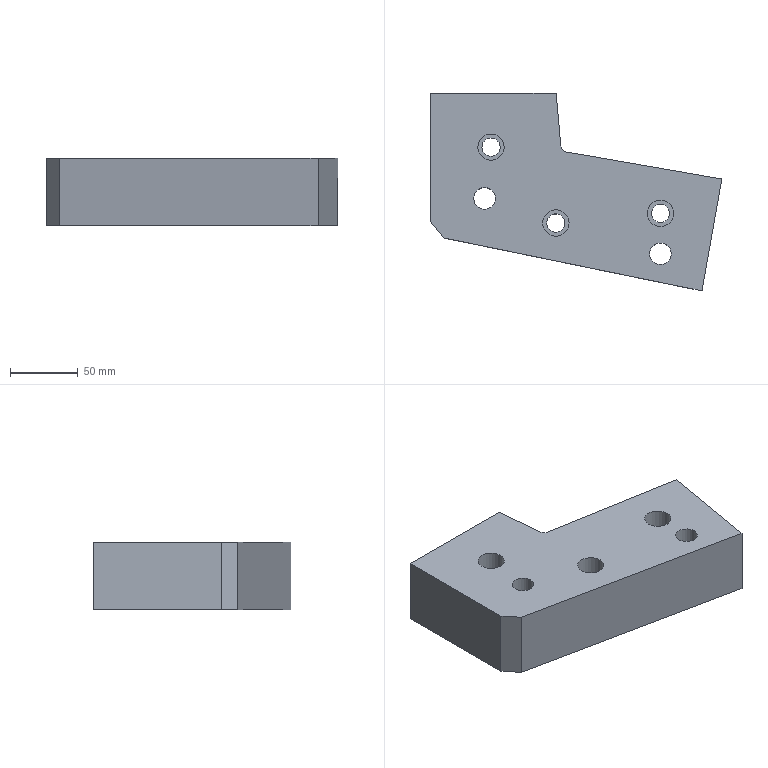Part | NX | features solid 2 | 1 solid | 25 faces | box 215.834 x 146.447 x 50 mm | volume 954922 mm3 | plane 13 | cylinder 10 | spline 2 | commonest cylinder face diameters 13.5 x3 19.5 x3 16 x2 10 x1 14 x1
STEP:
#1=CARTESIAN_POINT('',(903.262,333.786,0.));
#2=VERTEX_POINT('',#1);
#3=CARTESIAN_POINT('',(913.012,333.786,0.));
#4=DIRECTION('',(0.,0.,-1.));
#5=DIRECTION('',(-1.,0.,0.));
#6=AXIS2_PLACEMENT_3D('',#3,#4,#5);
#7=CIRCLE('',#6,9.75);
#8=EDGE_CURVE('',#2,#2,#7,.F.);
#9=ORIENTED_EDGE('',*,*,#8,.F.);
#10=EDGE_LOOP('',(#9));
#11=FACE_BOUND('',#10,.T.);
#12=CARTESIAN_POINT('',(829.797,322.775,0.));
#13=VERTEX_POINT('',#12);
#14=CARTESIAN_POINT('',(1021.231,283.553,0.));
#15=VERTEX_POINT('',#14);
#16=CARTESIAN_POINT('',(1017.086,284.403,0.));
#17=DIRECTION('',(0.9797,-0.2007,0.));
#18=VECTOR('',#17,1000.);
#19=LINE('',#16,#18);
#20=EDGE_CURVE('',#13,#15,#19,.T.);
#21=ORIENTED_EDGE('',*,*,#20,.T.);
#22=CARTESIAN_POINT('',(1035.834,366.376,0.));
#23=VERTEX_POINT('',#22);
#24=CARTESIAN_POINT('',(1025.414,307.279,0.));
#25=DIRECTION('',(0.1736,0.9848,0.));
#26=VECTOR('',#25,1000.);
#27=LINE('',#24,#26);
#28=EDGE_CURVE('',#15,#23,#27,.T.);
#29=ORIENTED_EDGE('',*,*,#28,.T.);
#30=CARTESIAN_POINT('',(920.475,386.408,0.));
#31=VERTEX_POINT('',#30);
#32=CARTESIAN_POINT('',(1323.576,316.335,0.));
#33=CARTESIAN_POINT('',(1303.952,319.748,0.));
#34=CARTESIAN_POINT('',(1284.328,323.16,0.));
#35=CARTESIAN_POINT('',(1264.704,326.573,0.));
#36=CARTESIAN_POINT('',(1233.889,331.932,0.));
#37=CARTESIAN_POINT('',(1172.258,342.651,0.));
#38=CARTESIAN_POINT('',(1095.22,356.049,0.));
#39=CARTESIAN_POINT('',(1033.589,366.767,0.));
#40=CARTESIAN_POINT('',(987.365,374.804,0.));
#41=CARTESIAN_POINT('',(948.847,381.509,0.));
#42=CARTESIAN_POINT('',(923.808,385.853,0.));
#43=CARTESIAN_POINT('',(914.109,387.486,0.));
#44=CARTESIAN_POINT('',(912.091,387.827,0.));
#45=CARTESIAN_POINT('',(911.971,387.848,0.));
#46=CARTESIAN_POINT('',(911.79,387.876,0.));
#47=CARTESIAN_POINT('',(911.394,387.917,0.));
#48=CARTESIAN_POINT('',(910.546,388.022,0.));
#49=CARTESIAN_POINT('',(908.847,388.221,0.));
#50=CARTESIAN_POINT('',(906.42,388.511,0.));
#51=CARTESIAN_POINT('',(903.994,388.799,0.));
#52=CARTESIAN_POINT('',(902.295,389.001,0.));
#53=CARTESIAN_POINT('',(901.446,389.101,0.));
#54=CARTESIAN_POINT('',(901.052,389.148,0.));
#55=CARTESIAN_POINT('',(900.87,389.17,0.));
#56=CARTESIAN_POINT('',(900.748,389.184,0.));
#57=CARTESIAN_POINT('',(899.68,389.239,0.));
#58=CARTESIAN_POINT('',(897.973,389.35,0.));
#59=CARTESIAN_POINT('',(896.023,389.486,0.));
#60=CARTESIAN_POINT('',(894.456,389.561,0.));
#61=CARTESIAN_POINT('',(892.989,389.903,0.));
#62=CARTESIAN_POINT('',(891.495,390.907,0.));
#63=CARTESIAN_POINT('',(890.458,392.378,0.));
#64=CARTESIAN_POINT('',(890.077,393.863,0.));
#65=CARTESIAN_POINT('',(889.825,397.101,0.));
#66=CARTESIAN_POINT('',(889.362,402.393,0.));
#67=CARTESIAN_POINT('',(888.928,407.354,0.));
#68=CARTESIAN_POINT('',(888.696,410.,0.));
#69=CARTESIAN_POINT('',(886.96,429.843,0.));
#70=CARTESIAN_POINT('',(885.224,449.685,0.));
#71=CARTESIAN_POINT('',(883.488,469.528,0.));
#72=B_SPLINE_CURVE_WITH_KNOTS('',3,(#32,#33,#34,#35,#36,#37,#38,#39,#40,#41,#42,#43,#44,#45,#46,#47,#48,#49,#50,#51,#52,#53,#54,#55,#56,#57,#58,#59,#60,#61,#62,#63,#64,#65,#66,#67,#68,#69,#70,#71),.UNSPECIFIED.,.F.,.F.,(4,3,1,1,1,1,1,1,1,1,1,1,1,1,1,1,1,1,1,1,1,1,1,1,1,1,1,1,1,1,1,1,3,4),(-0.15,0.,0.2355,0.4711,0.5889,0.7066,0.8244,0.8833,0.898,0.8985,0.8987,0.8989,0.8999,0.9017,0.9054,0.9127,0.9201,0.9238,0.9256,0.9265,0.9268,0.927,0.9275,0.9348,0.9399,0.9422,0.9466,0.9511,0.9555,0.96,0.9625,0.98,1.,1.15),.UNSPECIFIED.);
#73=EDGE_CURVE('',#23,#31,#72,.T.);
#74=ORIENTED_EDGE('',*,*,#73,.T.);
#75=CARTESIAN_POINT('',(916.651,390.837,0.));
#76=VERTEX_POINT('',#75);
#77=CARTESIAN_POINT('',(921.632,391.273,0.));
#78=DIRECTION('',(0.,0.,-1.));
#79=DIRECTION('',(-1.,0.,0.));
#80=AXIS2_PLACEMENT_3D('',#77,#78,#79);
#81=CIRCLE('',#80,5.);
#82=EDGE_CURVE('',#31,#76,#81,.T.);
#83=ORIENTED_EDGE('',*,*,#82,.T.);
#84=CARTESIAN_POINT('',(913.224,430.,0.));
#85=VERTEX_POINT('',#84);
#86=CARTESIAN_POINT('',(916.651,390.837,0.));
#87=DIRECTION('',(-0.08716,0.9962,0.));
#88=VECTOR('',#87,1000.);
#89=LINE('',#86,#88);
#90=EDGE_CURVE('',#76,#85,#89,.T.);
#91=ORIENTED_EDGE('',*,*,#90,.T.);
#92=CARTESIAN_POINT('',(820.,430.,0.));
#93=VERTEX_POINT('',#92);
#94=CARTESIAN_POINT('',(1021.9,430.,0.));
#95=DIRECTION('',(1.,0.,0.));
#96=VECTOR('',#95,1000.);
#97=LINE('',#94,#96);
#98=EDGE_CURVE('',#85,#93,#97,.F.);
#99=ORIENTED_EDGE('',*,*,#98,.T.);
#100=CARTESIAN_POINT('',(820.,334.782,0.));
#101=VERTEX_POINT('',#100);
#102=CARTESIAN_POINT('',(820.,410.,0.));
#103=DIRECTION('',(0.,-1.,0.));
#104=VECTOR('',#103,1000.);
#105=LINE('',#102,#104);
#106=EDGE_CURVE('',#93,#101,#105,.T.);
#107=ORIENTED_EDGE('',*,*,#106,.T.);
#108=CARTESIAN_POINT('',(820.,334.782,0.));
#109=DIRECTION('',(-0.6322,0.7748,0.));
#110=VECTOR('',#109,1000.);
#111=LINE('',#108,#110);
#112=EDGE_CURVE('',#101,#13,#111,.F.);
#113=ORIENTED_EDGE('',*,*,#112,.T.);
#114=EDGE_LOOP('',(#21,#29,#74,#83,#91,#99,#107,#113));
#115=FACE_BOUND('',#114,.T.);
#116=CARTESIAN_POINT('',(980.711,340.91,0.));
#117=VERTEX_POINT('',#116);
#118=CARTESIAN_POINT('',(990.461,340.91,0.));
#119=DIRECTION('',(0.,0.,-1.));
#120=DIRECTION('',(-1.,0.,0.));
#121=AXIS2_PLACEMENT_3D('',#118,#119,#120);
#122=CIRCLE('',#121,9.75);
#123=EDGE_CURVE('',#117,#117,#122,.F.);
#124=ORIENTED_EDGE('',*,*,#123,.F.);
#125=EDGE_LOOP('',(#124));
#126=FACE_BOUND('',#125,.T.);
#127=CARTESIAN_POINT('',(855.25,390.,0.));
#128=VERTEX_POINT('',#127);
#129=CARTESIAN_POINT('',(865.,390.,0.));
#130=DIRECTION('',(0.,0.,-1.));
#131=DIRECTION('',(-1.,0.,0.));
#132=AXIS2_PLACEMENT_3D('',#129,#130,#131);
#133=CIRCLE('',#132,9.75);
#134=EDGE_CURVE('',#128,#128,#133,.F.);
#135=ORIENTED_EDGE('',*,*,#134,.F.);
#136=EDGE_LOOP('',(#135));
#137=FACE_BOUND('',#136,.T.);
#138=CARTESIAN_POINT('',(852.203,352.007,0.));
#139=VERTEX_POINT('',#138);
#140=CARTESIAN_POINT('',(860.203,352.007,0.));
#141=DIRECTION('',(0.,0.,-1.));
#142=DIRECTION('',(-1.,0.,0.));
#143=AXIS2_PLACEMENT_3D('',#140,#141,#142);
#144=CIRCLE('',#143,8.);
#145=EDGE_CURVE('',#139,#139,#144,.F.);
#146=ORIENTED_EDGE('',*,*,#145,.F.);
#147=EDGE_LOOP('',(#146));
#148=FACE_BOUND('',#147,.T.);
#149=CARTESIAN_POINT('',(982.461,310.91,0.));
#150=VERTEX_POINT('',#149);
#151=CARTESIAN_POINT('',(990.461,310.91,0.));
#152=DIRECTION('',(0.,0.,-1.));
#153=DIRECTION('',(-1.,0.,0.));
#154=AXIS2_PLACEMENT_3D('',#151,#152,#153);
#155=CIRCLE('',#154,8.);
#156=EDGE_CURVE('',#150,#150,#155,.F.);
#157=ORIENTED_EDGE('',*,*,#156,.F.);
#158=EDGE_LOOP('',(#157));
#159=FACE_BOUND('',#158,.T.);
#160=CARTESIAN_POINT('',(1021.9,307.899,0.));
#161=DIRECTION('',(0.,0.,-1.));
#162=DIRECTION('',(1.,0.,0.));
#163=AXIS2_PLACEMENT_3D('',#160,#161,#162);
#164=PLANE('',#163);
#165=ADVANCED_FACE('',(#11,#115,#126,#137,#148,#159),#164,.F.);
#166=CARTESIAN_POINT('',(852.203,352.007,-50.));
#167=VERTEX_POINT('',#166);
#168=CARTESIAN_POINT('',(860.203,352.007,-50.));
#169=DIRECTION('',(0.,0.,-1.));
#170=DIRECTION('',(-1.,0.,0.));
#171=AXIS2_PLACEMENT_3D('',#168,#169,#170);
#172=CIRCLE('',#171,8.);
#173=EDGE_CURVE('',#167,#167,#172,.F.);
#174=ORIENTED_EDGE('',*,*,#173,.T.);
#175=EDGE_LOOP('',(#174));
#176=FACE_BOUND('',#175,.T.);
#177=CARTESIAN_POINT('',(858.25,390.,-50.));
#178=VERTEX_POINT('',#177);
#179=CARTESIAN_POINT('',(865.,390.,-50.));
#180=DIRECTION('',(0.,0.,-1.));
#181=DIRECTION('',(-1.,0.,0.));
#182=AXIS2_PLACEMENT_3D('',#179,#180,#181);
#183=CIRCLE('',#182,6.75);
#184=EDGE_CURVE('',#178,#178,#183,.F.);
#185=ORIENTED_EDGE('',*,*,#184,.T.);
#186=EDGE_LOOP('',(#185));
#187=FACE_BOUND('',#186,.T.);
#188=CARTESIAN_POINT('',(983.711,340.91,-50.));
#189=VERTEX_POINT('',#188);
#190=CARTESIAN_POINT('',(990.461,340.91,-50.));
#191=DIRECTION('',(0.,0.,-1.));
#192=DIRECTION('',(-1.,0.,0.));
#193=AXIS2_PLACEMENT_3D('',#190,#191,#192);
#194=CIRCLE('',#193,6.75);
#195=EDGE_CURVE('',#189,#189,#194,.F.);
#196=ORIENTED_EDGE('',*,*,#195,.T.);
#197=EDGE_LOOP('',(#196));
#198=FACE_BOUND('',#197,.T.);
#199=CARTESIAN_POINT('',(1021.231,283.553,-50.));
#200=VERTEX_POINT('',#199);
#201=CARTESIAN_POINT('',(1035.487,364.407,-50.));
#202=VERTEX_POINT('',#201);
#203=CARTESIAN_POINT('',(1025.414,307.279,-50.));
#204=DIRECTION('',(0.1736,0.9848,0.));
#205=VECTOR('',#204,1000.);
#206=LINE('',#203,#205);
#207=EDGE_CURVE('',#200,#202,#206,.T.);
#208=ORIENTED_EDGE('',*,*,#207,.F.);
#209=CARTESIAN_POINT('',(829.797,322.775,-50.));
#210=VERTEX_POINT('',#209);
#211=CARTESIAN_POINT('',(1017.086,284.403,-50.));
#212=DIRECTION('',(0.9797,-0.2007,0.));
#213=VECTOR('',#212,1000.);
#214=LINE('',#211,#213);
#215=EDGE_CURVE('',#210,#200,#214,.T.);
#216=ORIENTED_EDGE('',*,*,#215,.F.);
#217=CARTESIAN_POINT('',(820.,334.782,-50.));
#218=VERTEX_POINT('',#217);
#219=CARTESIAN_POINT('',(913.856,219.747,-50.));
#220=DIRECTION('',(0.6322,-0.7748,0.));
#221=VECTOR('',#220,1000.);
#222=LINE('',#219,#221);
#223=EDGE_CURVE('',#210,#218,#222,.F.);
#224=ORIENTED_EDGE('',*,*,#223,.T.);
#225=CARTESIAN_POINT('',(820.,430.,-50.));
#226=VERTEX_POINT('',#225);
#227=CARTESIAN_POINT('',(820.,410.,-50.));
#228=DIRECTION('',(0.,-1.,0.));
#229=VECTOR('',#228,1000.);
#230=LINE('',#227,#229);
#231=EDGE_CURVE('',#226,#218,#230,.T.);
#232=ORIENTED_EDGE('',*,*,#231,.F.);
#233=CARTESIAN_POINT('',(911.217,430.,-50.));
#234=VERTEX_POINT('',#233);
#235=CARTESIAN_POINT('',(1021.9,430.,-50.));
#236=DIRECTION('',(1.,0.,0.));
#237=VECTOR('',#236,1000.);
#238=LINE('',#235,#237);
#239=EDGE_CURVE('',#234,#226,#238,.F.);
#240=ORIENTED_EDGE('',*,*,#239,.F.);
#241=CARTESIAN_POINT('',(914.658,390.663,-50.));
#242=VERTEX_POINT('',#241);
#243=CARTESIAN_POINT('',(914.658,390.663,-50.));
#244=DIRECTION('',(-0.08716,0.9962,0.));
#245=VECTOR('',#244,1000.);
#246=LINE('',#243,#245);
#247=EDGE_CURVE('',#242,#234,#246,.T.);
#248=ORIENTED_EDGE('',*,*,#247,.F.);
#249=CARTESIAN_POINT('',(920.081,384.447,-50.));
#250=VERTEX_POINT('',#249);
#251=CARTESIAN_POINT('',(921.632,391.273,-50.));
#252=DIRECTION('',(0.,0.,-1.));
#253=DIRECTION('',(-1.,0.,0.));
#254=AXIS2_PLACEMENT_3D('',#251,#252,#253);
#255=CIRCLE('',#254,7.);
#256=EDGE_CURVE('',#250,#242,#255,.T.);
#257=ORIENTED_EDGE('',*,*,#256,.F.);
#258=CARTESIAN_POINT('',(920.081,384.447,-50.));
#259=CARTESIAN_POINT('',(920.552,384.367,-50.));
#260=CARTESIAN_POINT('',(921.288,384.241,-50.));
#261=CARTESIAN_POINT('',(922.185,384.088,-50.));
#262=CARTESIAN_POINT('',(922.726,383.995,-50.));
#263=CARTESIAN_POINT('',(923.034,383.943,-50.));
#264=CARTESIAN_POINT('',(923.367,383.886,-50.));
#265=CARTESIAN_POINT('',(923.396,383.881,-50.));
#266=CARTESIAN_POINT('',(923.576,383.85,-50.));
#267=CARTESIAN_POINT('',(923.851,383.803,-50.));
#268=CARTESIAN_POINT('',(924.31,383.724,-50.));
#269=CARTESIAN_POINT('',(924.87,383.628,-50.));
#270=CARTESIAN_POINT('',(925.66,383.492,-50.));
#271=CARTESIAN_POINT('',(926.718,383.31,-50.));
#272=CARTESIAN_POINT('',(928.103,383.072,-50.));
#273=CARTESIAN_POINT('',(930.103,382.726,-50.));
#274=CARTESIAN_POINT('',(932.889,382.245,-50.));
#275=CARTESIAN_POINT('',(936.692,381.586,-50.));
#276=CARTESIAN_POINT('',(940.241,380.97,-50.));
#277=CARTESIAN_POINT('',(943.314,380.437,-50.));
#278=CARTESIAN_POINT('',(945.322,380.088,-50.));
#279=CARTESIAN_POINT('',(946.793,379.833,-50.));
#280=CARTESIAN_POINT('',(947.521,379.706,-50.));
#281=CARTESIAN_POINT('',(947.972,379.628,-50.));
#282=CARTESIAN_POINT('',(948.365,379.56,-50.));
#283=CARTESIAN_POINT('',(949.073,379.437,-50.));
#284=CARTESIAN_POINT('',(950.244,379.233,-50.));
#285=CARTESIAN_POINT('',(951.737,378.974,-50.));
#286=CARTESIAN_POINT('',(954.11,378.561,-50.));
#287=CARTESIAN_POINT('',(957.082,378.045,-50.));
#288=CARTESIAN_POINT('',(960.645,377.425,-50.));
#289=CARTESIAN_POINT('',(965.397,376.599,-50.));
#290=CARTESIAN_POINT('',(971.337,375.567,-50.));
#291=CARTESIAN_POINT('',(978.465,374.327,-50.));
#292=CARTESIAN_POINT('',(985.593,373.088,-50.));
#293=CARTESIAN_POINT('',(995.097,371.435,-50.));
#294=CARTESIAN_POINT('',(1006.976,369.369,-50.));
#295=CARTESIAN_POINT('',(1021.232,366.889,-50.));
#296=CARTESIAN_POINT('',(1030.736,365.235,-50.));
#297=CARTESIAN_POINT('',(1035.487,364.408,-50.));
#298=B_SPLINE_CURVE_WITH_KNOTS('',3,(#258,#259,#260,#261,#262,#263,#264,#265,#266,#267,#268,#269,#270,#271,#272,#273,#274,#275,#276,#277,#278,#279,#280,#281,#282,#283,#284,#285,#286,#287,#288,#289,#290,#291,#292,#293,#294,#295,#296,#297),.UNSPECIFIED.,.F.,.F.,(4,1,1,1,1,1,1,1,1,1,1,1,1,1,1,1,1,1,1,1,1,1,1,1,1,1,1,1,1,1,1,1,1,1,1,1,1,4),(0.1827,0.1849,0.1861,0.1866,0.1872,0.1875,0.1878,0.1883,0.1895,0.1917,0.194,0.1963,0.2008,0.2053,0.2099,0.2189,0.228,0.237,0.2416,0.2461,0.2484,0.2495,0.2501,0.2506,0.2529,0.2551,0.2597,0.2642,0.2733,0.2823,0.2914,0.3095,0.3276,0.3457,0.3639,0.4001,0.4363,0.4726),.UNSPECIFIED.);
#299=EDGE_CURVE('',#202,#250,#298,.F.);
#300=ORIENTED_EDGE('',*,*,#299,.F.);
#301=EDGE_LOOP('',(#208,#216,#224,#232,#240,#248,#257,#300));
#302=FACE_BOUND('',#301,.T.);
#303=CARTESIAN_POINT('',(906.262,333.786,-50.));
#304=VERTEX_POINT('',#303);
#305=CARTESIAN_POINT('',(913.012,333.786,-50.));
#306=DIRECTION('',(0.,0.,-1.));
#307=DIRECTION('',(-1.,0.,0.));
#308=AXIS2_PLACEMENT_3D('',#305,#306,#307);
#309=CIRCLE('',#308,6.75);
#310=EDGE_CURVE('',#304,#304,#309,.T.);
#311=ORIENTED_EDGE('',*,*,#310,.F.);
#312=EDGE_LOOP('',(#311));
#313=FACE_BOUND('',#312,.T.);
#314=CARTESIAN_POINT('',(982.461,310.91,-50.));
#315=VERTEX_POINT('',#314);
#316=CARTESIAN_POINT('',(990.461,310.91,-50.));
#317=DIRECTION('',(0.,0.,-1.));
#318=DIRECTION('',(-1.,0.,0.));
#319=AXIS2_PLACEMENT_3D('',#316,#317,#318);
#320=CIRCLE('',#319,8.);
#321=EDGE_CURVE('',#315,#315,#320,.F.);
#322=ORIENTED_EDGE('',*,*,#321,.T.);
#323=EDGE_LOOP('',(#322));
#324=FACE_BOUND('',#323,.T.);
#325=CARTESIAN_POINT('',(1021.9,307.899,-50.));
#326=DIRECTION('',(0.,0.,-1.));
#327=DIRECTION('',(1.,0.,0.));
#328=AXIS2_PLACEMENT_3D('',#325,#326,#327);
#329=PLANE('',#328);
#330=ADVANCED_FACE('',(#176,#187,#198,#302,#313,#324),#329,.T.);
#331=ORIENTED_EDGE('',*,*,#310,.T.);
#332=EDGE_LOOP('',(#331));
#333=FACE_BOUND('',#332,.T.);
#334=CARTESIAN_POINT('',(919.762,333.786,-25.));
#335=VERTEX_POINT('',#334);
#336=CARTESIAN_POINT('',(913.012,333.786,-25.));
#337=DIRECTION('',(0.,0.,1.));
#338=DIRECTION('',(1.,0.,0.));
#339=AXIS2_PLACEMENT_3D('',#336,#337,#338);
#340=CIRCLE('',#339,6.75);
#341=EDGE_CURVE('',#335,#335,#340,.F.);
#342=ORIENTED_EDGE('',*,*,#341,.F.);
#343=EDGE_LOOP('',(#342));
#344=FACE_BOUND('',#343,.T.);
#345=CARTESIAN_POINT('',(913.012,333.786,-15.));
#346=DIRECTION('',(0.,0.,-1.));
#347=DIRECTION('',(-1.,0.,0.));
#348=AXIS2_PLACEMENT_3D('',#345,#346,#347);
#349=CYLINDRICAL_SURFACE('',#348,6.75);
#350=ADVANCED_FACE('',(#333,#344),#349,.F.);
#351=CARTESIAN_POINT('',(874.75,390.,-25.));
#352=VERTEX_POINT('',#351);
#353=CARTESIAN_POINT('',(865.,390.,-25.));
#354=DIRECTION('',(0.,0.,1.));
#355=DIRECTION('',(1.,0.,0.));
#356=AXIS2_PLACEMENT_3D('',#353,#354,#355);
#357=CIRCLE('',#356,9.75);
#358=EDGE_CURVE('',#352,#352,#357,.T.);
#359=ORIENTED_EDGE('',*,*,#358,.T.);
#360=EDGE_LOOP('',(#359));
#361=FACE_BOUND('',#360,.T.);
#362=CARTESIAN_POINT('',(871.75,390.,-25.));
#363=VERTEX_POINT('',#362);
#364=CARTESIAN_POINT('',(865.,390.,-25.));
#365=DIRECTION('',(0.,0.,1.));
#366=DIRECTION('',(1.,0.,0.));
#367=AXIS2_PLACEMENT_3D('',#364,#365,#366);
#368=CIRCLE('',#367,6.75);
#369=EDGE_CURVE('',#363,#363,#368,.F.);
#370=ORIENTED_EDGE('',*,*,#369,.T.);
#371=EDGE_LOOP('',(#370));
#372=FACE_BOUND('',#371,.T.);
#373=CARTESIAN_POINT('',(865.,390.,-25.));
#374=DIRECTION('',(0.,0.,1.));
#375=DIRECTION('',(1.,0.,0.));
#376=AXIS2_PLACEMENT_3D('',#373,#374,#375);
#377=PLANE('',#376);
#378=ADVANCED_FACE('',(#361,#372),#377,.T.);
#379=CARTESIAN_POINT('',(1000.211,340.91,-25.));
#380=VERTEX_POINT('',#379);
#381=CARTESIAN_POINT('',(990.461,340.91,-25.));
#382=DIRECTION('',(0.,0.,1.));
#383=DIRECTION('',(1.,0.,0.));
#384=AXIS2_PLACEMENT_3D('',#381,#382,#383);
#385=CIRCLE('',#384,9.75);
#386=EDGE_CURVE('',#380,#380,#385,.T.);
#387=ORIENTED_EDGE('',*,*,#386,.T.);
#388=EDGE_LOOP('',(#387));
#389=FACE_BOUND('',#388,.T.);
#390=CARTESIAN_POINT('',(997.211,340.91,-25.));
#391=VERTEX_POINT('',#390);
#392=CARTESIAN_POINT('',(990.461,340.91,-25.));
#393=DIRECTION('',(0.,0.,1.));
#394=DIRECTION('',(1.,0.,0.));
#395=AXIS2_PLACEMENT_3D('',#392,#393,#394);
#396=CIRCLE('',#395,6.75);
#397=EDGE_CURVE('',#391,#391,#396,.F.);
#398=ORIENTED_EDGE('',*,*,#397,.T.);
#399=EDGE_LOOP('',(#398));
#400=FACE_BOUND('',#399,.T.);
#401=CARTESIAN_POINT('',(990.461,340.91,-25.));
#402=DIRECTION('',(0.,0.,1.));
#403=DIRECTION('',(1.,0.,0.));
#404=AXIS2_PLACEMENT_3D('',#401,#402,#403);
#405=PLANE('',#404);
#406=ADVANCED_FACE('',(#389,#400),#405,.T.);
#407=ORIENTED_EDGE('',*,*,#184,.F.);
#408=EDGE_LOOP('',(#407));
#409=FACE_BOUND('',#408,.T.);
#410=ORIENTED_EDGE('',*,*,#369,.F.);
#411=EDGE_LOOP('',(#410));
#412=FACE_BOUND('',#411,.T.);
#413=CARTESIAN_POINT('',(865.,390.,75.));
#414=DIRECTION('',(0.,0.,-1.));
#415=DIRECTION('',(-1.,0.,0.));
#416=AXIS2_PLACEMENT_3D('',#413,#414,#415);
#417=CYLINDRICAL_SURFACE('',#416,6.75);
#418=ADVANCED_FACE('',(#409,#412),#417,.F.);
#419=ORIENTED_EDGE('',*,*,#195,.F.);
#420=EDGE_LOOP('',(#419));
#421=FACE_BOUND('',#420,.T.);
#422=ORIENTED_EDGE('',*,*,#397,.F.);
#423=EDGE_LOOP('',(#422));
#424=FACE_BOUND('',#423,.T.);
#425=CARTESIAN_POINT('',(990.461,340.91,75.));
#426=DIRECTION('',(0.,0.,-1.));
#427=DIRECTION('',(-1.,0.,0.));
#428=AXIS2_PLACEMENT_3D('',#425,#426,#427);
#429=CYLINDRICAL_SURFACE('',#428,6.75);
#430=ADVANCED_FACE('',(#421,#424),#429,.F.);
#431=ORIENTED_EDGE('',*,*,#173,.F.);
#432=EDGE_LOOP('',(#431));
#433=FACE_BOUND('',#432,.T.);
#434=ORIENTED_EDGE('',*,*,#145,.T.);
#435=EDGE_LOOP('',(#434));
#436=FACE_BOUND('',#435,.T.);
#437=CARTESIAN_POINT('',(860.203,352.007,50.));
#438=DIRECTION('',(0.,0.,-1.));
#439=DIRECTION('',(-1.,0.,0.));
#440=AXIS2_PLACEMENT_3D('',#437,#438,#439);
#441=CYLINDRICAL_SURFACE('',#440,8.);
#442=ADVANCED_FACE('',(#433,#436),#441,.F.);
#443=ORIENTED_EDGE('',*,*,#358,.F.);
#444=EDGE_LOOP('',(#443));
#445=FACE_BOUND('',#444,.T.);
#446=ORIENTED_EDGE('',*,*,#134,.T.);
#447=EDGE_LOOP('',(#446));
#448=FACE_BOUND('',#447,.T.);
#449=CARTESIAN_POINT('',(865.,390.,75.));
#450=DIRECTION('',(0.,0.,-1.));
#451=DIRECTION('',(-1.,0.,0.));
#452=AXIS2_PLACEMENT_3D('',#449,#450,#451);
#453=CYLINDRICAL_SURFACE('',#452,9.75);
#454=ADVANCED_FACE('',(#445,#448),#453,.F.);
#455=ORIENTED_EDGE('',*,*,#386,.F.);
#456=EDGE_LOOP('',(#455));
#457=FACE_BOUND('',#456,.T.);
#458=ORIENTED_EDGE('',*,*,#123,.T.);
#459=EDGE_LOOP('',(#458));
#460=FACE_BOUND('',#459,.T.);
#461=CARTESIAN_POINT('',(990.461,340.91,75.));
#462=DIRECTION('',(0.,0.,-1.));
#463=DIRECTION('',(-1.,0.,0.));
#464=AXIS2_PLACEMENT_3D('',#461,#462,#463);
#465=CYLINDRICAL_SURFACE('',#464,9.75);
#466=ADVANCED_FACE('',(#457,#460),#465,.F.);
#467=ORIENTED_EDGE('',*,*,#231,.T.);
#468=CARTESIAN_POINT('',(820.,334.782,-50.));
#469=DIRECTION('',(0.,0.,1.));
#470=VECTOR('',#469,1000.);
#471=LINE('',#468,#470);
#472=EDGE_CURVE('',#218,#101,#471,.T.);
#473=ORIENTED_EDGE('',*,*,#472,.T.);
#474=ORIENTED_EDGE('',*,*,#106,.F.);
#475=CARTESIAN_POINT('',(820.,430.,-50.));
#476=DIRECTION('',(0.,0.,-1.));
#477=VECTOR('',#476,1000.);
#478=LINE('',#475,#477);
#479=EDGE_CURVE('',#226,#93,#478,.F.);
#480=ORIENTED_EDGE('',*,*,#479,.F.);
#481=EDGE_LOOP('',(#467,#473,#474,#480));
#482=FACE_BOUND('',#481,.T.);
#483=CARTESIAN_POINT('',(820.,410.,-50.));
#484=DIRECTION('',(1.,0.,0.));
#485=DIRECTION('',(0.,-1.,0.));
#486=AXIS2_PLACEMENT_3D('',#483,#484,#485);
#487=PLANE('',#486);
#488=ADVANCED_FACE('',(#482),#487,.F.);
#489=CARTESIAN_POINT('',(916.651,390.837,-15.));
#490=VERTEX_POINT('',#489);
#491=CARTESIAN_POINT('',(916.651,390.837,-50.));
#492=DIRECTION('',(0.,0.,1.));
#493=VECTOR('',#492,1000.);
#494=LINE('',#491,#493);
#495=EDGE_CURVE('',#490,#76,#494,.T.);
#496=ORIENTED_EDGE('',*,*,#495,.T.);
#497=ORIENTED_EDGE('',*,*,#82,.F.);
#498=CARTESIAN_POINT('',(920.475,386.408,-15.));
#499=VERTEX_POINT('',#498);
#500=CARTESIAN_POINT('',(920.475,386.408,-7.5));
#501=DIRECTION('',(0.,0.,1.));
#502=VECTOR('',#501,1000.);
#503=LINE('',#500,#502);
#504=EDGE_CURVE('',#31,#499,#503,.F.);
#505=ORIENTED_EDGE('',*,*,#504,.T.);
#506=CARTESIAN_POINT('',(921.632,391.273,-15.));
#507=DIRECTION('',(0.,0.,-1.));
#508=DIRECTION('',(-1.,0.,0.));
#509=AXIS2_PLACEMENT_3D('',#506,#507,#508);
#510=CIRCLE('',#509,5.);
#511=EDGE_CURVE('',#499,#490,#510,.T.);
#512=ORIENTED_EDGE('',*,*,#511,.T.);
#513=EDGE_LOOP('',(#496,#497,#505,#512));
#514=FACE_BOUND('',#513,.T.);
#515=CARTESIAN_POINT('',(921.632,391.273,-50.));
#516=DIRECTION('',(0.,0.,1.));
#517=DIRECTION('',(-1.,0.,0.));
#518=AXIS2_PLACEMENT_3D('',#515,#516,#517);
#519=CYLINDRICAL_SURFACE('',#518,5.);
#520=ADVANCED_FACE('',(#514),#519,.F.);
#521=CARTESIAN_POINT('',(913.224,430.,-15.));
#522=VERTEX_POINT('',#521);
#523=CARTESIAN_POINT('',(913.224,430.,-50.));
#524=DIRECTION('',(0.,0.,1.));
#525=VECTOR('',#524,1000.);
#526=LINE('',#523,#525);
#527=EDGE_CURVE('',#522,#85,#526,.T.);
#528=ORIENTED_EDGE('',*,*,#527,.T.);
#529=ORIENTED_EDGE('',*,*,#90,.F.);
#530=ORIENTED_EDGE('',*,*,#495,.F.);
#531=CARTESIAN_POINT('',(916.651,390.837,-15.));
#532=DIRECTION('',(-0.08716,0.9962,0.));
#533=VECTOR('',#532,1000.);
#534=LINE('',#531,#533);
#535=EDGE_CURVE('',#490,#522,#534,.T.);
#536=ORIENTED_EDGE('',*,*,#535,.T.);
#537=EDGE_LOOP('',(#528,#529,#530,#536));
#538=FACE_BOUND('',#537,.T.);
#539=CARTESIAN_POINT('',(916.651,390.837,-50.));
#540=DIRECTION('',(-0.9962,-0.08716,0.));
#541=DIRECTION('',(-0.08716,0.9962,0.));
#542=AXIS2_PLACEMENT_3D('',#539,#540,#541);
#543=PLANE('',#542);
#544=ADVANCED_FACE('',(#538),#543,.F.);
#545=ORIENTED_EDGE('',*,*,#98,.F.);
#546=ORIENTED_EDGE('',*,*,#527,.F.);
#547=CARTESIAN_POINT('',(911.217,430.,-15.));
#548=VERTEX_POINT('',#547);
#549=CARTESIAN_POINT('',(872.888,430.,-15.));
#550=DIRECTION('',(1.,0.,0.));
#551=VECTOR('',#550,1000.);
#552=LINE('',#549,#551);
#553=EDGE_CURVE('',#522,#548,#552,.F.);
#554=ORIENTED_EDGE('',*,*,#553,.T.);
#555=CARTESIAN_POINT('',(911.217,430.,-50.));
#556=DIRECTION('',(0.,0.,1.));
#557=VECTOR('',#556,1000.);
#558=LINE('',#555,#557);
#559=EDGE_CURVE('',#234,#548,#558,.T.);
#560=ORIENTED_EDGE('',*,*,#559,.F.);
#561=ORIENTED_EDGE('',*,*,#239,.T.);
#562=ORIENTED_EDGE('',*,*,#479,.T.);
#563=EDGE_LOOP('',(#545,#546,#554,#560,#561,#562));
#564=FACE_BOUND('',#563,.T.);
#565=CARTESIAN_POINT('',(752.827,430.,-50.));
#566=DIRECTION('',(0.,1.,0.));
#567=DIRECTION('',(1.,0.,0.));
#568=AXIS2_PLACEMENT_3D('',#565,#566,#567);
#569=PLANE('',#568);
#570=ADVANCED_FACE('',(#564),#569,.T.);
#571=CARTESIAN_POINT('',(914.658,390.663,-15.));
#572=VERTEX_POINT('',#571);
#573=CARTESIAN_POINT('',(914.658,390.663,-15.));
#574=DIRECTION('',(-0.08716,0.9962,0.));
#575=VECTOR('',#574,1000.);
#576=LINE('',#573,#575);
#577=EDGE_CURVE('',#572,#548,#576,.T.);
#578=ORIENTED_EDGE('',*,*,#577,.F.);
#579=CARTESIAN_POINT('',(914.658,390.663,-50.));
#580=DIRECTION('',(0.,0.,1.));
#581=VECTOR('',#580,1000.);
#582=LINE('',#579,#581);
#583=EDGE_CURVE('',#242,#572,#582,.T.);
#584=ORIENTED_EDGE('',*,*,#583,.F.);
#585=ORIENTED_EDGE('',*,*,#247,.T.);
#586=ORIENTED_EDGE('',*,*,#559,.T.);
#587=EDGE_LOOP('',(#578,#584,#585,#586));
#588=FACE_BOUND('',#587,.T.);
#589=CARTESIAN_POINT('',(914.658,390.663,-50.));
#590=DIRECTION('',(-0.9962,-0.08716,0.));
#591=DIRECTION('',(-0.08716,0.9962,0.));
#592=AXIS2_PLACEMENT_3D('',#589,#590,#591);
#593=PLANE('',#592);
#594=ADVANCED_FACE('',(#588),#593,.F.);
#595=CARTESIAN_POINT('',(920.081,384.447,-15.));
#596=VERTEX_POINT('',#595);
#597=CARTESIAN_POINT('',(921.632,391.273,-15.));
#598=DIRECTION('',(0.,0.,-1.));
#599=DIRECTION('',(-1.,0.,0.));
#600=AXIS2_PLACEMENT_3D('',#597,#598,#599);
#601=CIRCLE('',#600,7.);
#602=EDGE_CURVE('',#596,#572,#601,.T.);
#603=ORIENTED_EDGE('',*,*,#602,.F.);
#604=CARTESIAN_POINT('',(920.081,384.447,-32.5));
#605=DIRECTION('',(0.,0.,1.));
#606=VECTOR('',#605,1000.);
#607=LINE('',#604,#606);
#608=EDGE_CURVE('',#596,#250,#607,.F.);
#609=ORIENTED_EDGE('',*,*,#608,.T.);
#610=ORIENTED_EDGE('',*,*,#256,.T.);
#611=ORIENTED_EDGE('',*,*,#583,.T.);
#612=EDGE_LOOP('',(#603,#609,#610,#611));
#613=FACE_BOUND('',#612,.T.);
#614=CARTESIAN_POINT('',(921.632,391.273,-50.));
#615=DIRECTION('',(0.,0.,1.));
#616=DIRECTION('',(-1.,0.,0.));
#617=AXIS2_PLACEMENT_3D('',#614,#615,#616);
#618=CYLINDRICAL_SURFACE('',#617,7.);
#619=ADVANCED_FACE('',(#613),#618,.F.);
#620=ORIENTED_EDGE('',*,*,#223,.F.);
#621=CARTESIAN_POINT('',(829.797,322.775,-50.));
#622=DIRECTION('',(0.,0.,-1.));
#623=VECTOR('',#622,1000.);
#624=LINE('',#621,#623);
#625=EDGE_CURVE('',#13,#210,#624,.T.);
#626=ORIENTED_EDGE('',*,*,#625,.F.);
#627=ORIENTED_EDGE('',*,*,#112,.F.);
#628=ORIENTED_EDGE('',*,*,#472,.F.);
#629=EDGE_LOOP('',(#620,#626,#627,#628));
#630=FACE_BOUND('',#629,.T.);
#631=CARTESIAN_POINT('',(820.,334.782,-50.));
#632=DIRECTION('',(0.7748,0.6322,0.));
#633=DIRECTION('',(-0.6322,0.7748,0.));
#634=AXIS2_PLACEMENT_3D('',#631,#632,#633);
#635=PLANE('',#634);
#636=ADVANCED_FACE('',(#630),#635,.F.);
#637=CARTESIAN_POINT('',(1035.834,366.376,-15.));
#638=VERTEX_POINT('',#637);
#639=CARTESIAN_POINT('',(982.86,375.59,-15.));
#640=VERTEX_POINT('',#639);
#641=CARTESIAN_POINT('',(982.86,375.59,-15.));
#642=CARTESIAN_POINT('',(989.501,374.434,-15.));
#643=CARTESIAN_POINT('',(1007.159,371.363,-15.));
#644=CARTESIAN_POINT('',(1035.834,366.376,-15.));
#645=B_SPLINE_CURVE_WITH_KNOTS('',3,(#641,#642,#643,#644),.UNSPECIFIED.,.F.,.F.,(4,4),(0.,0.9049),.UNSPECIFIED.);
#646=EDGE_CURVE('',#638,#640,#645,.F.);
#647=ORIENTED_EDGE('',*,*,#646,.F.);
#648=CARTESIAN_POINT('',(1035.487,364.406,-15.));
#649=VERTEX_POINT('',#648);
#650=CARTESIAN_POINT('',(1022.389,290.122,-15.));
#651=DIRECTION('',(0.1736,0.9848,0.));
#652=VECTOR('',#651,1000.);
#653=LINE('',#650,#652);
#654=EDGE_CURVE('',#638,#649,#653,.F.);
#655=ORIENTED_EDGE('',*,*,#654,.T.);
#656=CARTESIAN_POINT('',(920.081,384.447,-15.));
#657=CARTESIAN_POINT('',(939.326,381.172,-15.));
#658=CARTESIAN_POINT('',(977.783,374.423,-15.));
#659=CARTESIAN_POINT('',(1016.253,367.751,-15.));
#660=CARTESIAN_POINT('',(1035.487,364.406,-15.));
#661=B_SPLINE_CURVE_WITH_KNOTS('',3,(#656,#657,#658,#659,#660),.UNSPECIFIED.,.F.,.F.,(4,1,4),(0.6912,0.7497,0.8083),.UNSPECIFIED.);
#662=EDGE_CURVE('',#649,#596,#661,.F.);
#663=ORIENTED_EDGE('',*,*,#662,.T.);
#664=ORIENTED_EDGE('',*,*,#602,.T.);
#665=ORIENTED_EDGE('',*,*,#577,.T.);
#666=ORIENTED_EDGE('',*,*,#553,.F.);
#667=ORIENTED_EDGE('',*,*,#535,.F.);
#668=ORIENTED_EDGE('',*,*,#511,.F.);
#669=CARTESIAN_POINT('',(982.86,375.59,-15.));
#670=CARTESIAN_POINT('',(962.067,379.207,-15.));
#671=CARTESIAN_POINT('',(941.281,382.867,-15.));
#672=CARTESIAN_POINT('',(920.475,386.408,-15.));
#673=B_SPLINE_CURVE_WITH_KNOTS('',3,(#669,#670,#671,#672),.UNSPECIFIED.,.F.,.F.,(4,4),(-0.009288,0.05403),.UNSPECIFIED.);
#674=EDGE_CURVE('',#640,#499,#673,.T.);
#675=ORIENTED_EDGE('',*,*,#674,.F.);
#676=EDGE_LOOP('',(#647,#655,#663,#664,#665,#666,#667,#668,#675));
#677=FACE_BOUND('',#676,.T.);
#678=CARTESIAN_POINT('',(1245.,250.87,-15.));
#679=DIRECTION('',(0.,0.,-1.));
#680=DIRECTION('',(0.,1.,0.));
#681=AXIS2_PLACEMENT_3D('',#678,#679,#680);
#682=PLANE('',#681);
#683=ADVANCED_FACE('',(#677),#682,.T.);
#684=ORIENTED_EDGE('',*,*,#73,.F.);
#685=CARTESIAN_POINT('',(1035.834,366.376,-7.5));
#686=DIRECTION('',(0.,0.,1.));
#687=VECTOR('',#686,1000.);
#688=LINE('',#685,#687);
#689=EDGE_CURVE('',#23,#638,#688,.F.);
#690=ORIENTED_EDGE('',*,*,#689,.T.);
#691=ORIENTED_EDGE('',*,*,#646,.T.);
#692=ORIENTED_EDGE('',*,*,#674,.T.);
#693=ORIENTED_EDGE('',*,*,#504,.F.);
#694=EDGE_LOOP('',(#684,#690,#691,#692,#693));
#695=FACE_BOUND('',#694,.T.);
#696=CARTESIAN_POINT('',(1035.834,366.376,-15.));
#697=CARTESIAN_POINT('',(1035.834,366.376,0.));
#698=CARTESIAN_POINT('',(1016.609,369.719,-15.));
#699=CARTESIAN_POINT('',(1016.609,369.719,0.));
#700=CARTESIAN_POINT('',(978.154,376.389,-15.));
#701=CARTESIAN_POINT('',(978.154,376.389,0.));
#702=CARTESIAN_POINT('',(939.712,383.134,-15.));
#703=CARTESIAN_POINT('',(939.712,383.134,0.));
#704=CARTESIAN_POINT('',(920.475,386.408,-15.));
#705=CARTESIAN_POINT('',(920.475,386.408,0.));
#706=B_SPLINE_SURFACE_WITH_KNOTS('',3,1,((#696,#697),(#698,#699),(#700,#701),(#702,#703),(#704,#705)),.SURF_OF_LINEAR_EXTRUSION.,.F.,.F.,.F.,(4,1,4),(2,2),(0.5831,0.7301,0.8771),(0.,1.),.UNSPECIFIED.);
#707=ADVANCED_FACE('',(#695),#706,.T.);
#708=ORIENTED_EDGE('',*,*,#662,.F.);
#709=CARTESIAN_POINT('',(1035.487,364.406,-32.5));
#710=DIRECTION('',(0.,0.,1.));
#711=VECTOR('',#710,1000.);
#712=LINE('',#709,#711);
#713=EDGE_CURVE('',#649,#202,#712,.F.);
#714=ORIENTED_EDGE('',*,*,#713,.T.);
#715=ORIENTED_EDGE('',*,*,#299,.T.);
#716=ORIENTED_EDGE('',*,*,#608,.F.);
#717=EDGE_LOOP('',(#708,#714,#715,#716));
#718=FACE_BOUND('',#717,.T.);
#719=CARTESIAN_POINT('',(1035.487,364.406,-50.));
#720=CARTESIAN_POINT('',(1035.487,364.406,-15.));
#721=CARTESIAN_POINT('',(1016.252,367.751,-50.));
#722=CARTESIAN_POINT('',(1016.252,367.751,-15.));
#723=CARTESIAN_POINT('',(977.782,374.423,-50.));
#724=CARTESIAN_POINT('',(977.782,374.423,-15.));
#725=CARTESIAN_POINT('',(939.315,381.173,-50.));
#726=CARTESIAN_POINT('',(939.315,381.173,-15.));
#727=CARTESIAN_POINT('',(920.081,384.447,-50.));
#728=CARTESIAN_POINT('',(920.081,384.447,-15.));
#729=B_SPLINE_SURFACE_WITH_KNOTS('',3,1,((#719,#720),(#721,#722),(#723,#724),(#725,#726),(#727,#728)),.SURF_OF_LINEAR_EXTRUSION.,.F.,.F.,.F.,(4,1,4),(2,2),(0.5817,0.7293,0.8768),(0.,1.),.UNSPECIFIED.);
#730=ADVANCED_FACE('',(#718),#729,.T.);
#731=ORIENTED_EDGE('',*,*,#215,.T.);
#732=CARTESIAN_POINT('',(1021.231,283.553,-50.));
#733=DIRECTION('',(0.,0.,1.));
#734=VECTOR('',#733,1000.);
#735=LINE('',#732,#734);
#736=EDGE_CURVE('',#200,#15,#735,.T.);
#737=ORIENTED_EDGE('',*,*,#736,.T.);
#738=ORIENTED_EDGE('',*,*,#20,.F.);
#739=ORIENTED_EDGE('',*,*,#625,.T.);
#740=EDGE_LOOP('',(#731,#737,#738,#739));
#741=FACE_BOUND('',#740,.T.);
#742=CARTESIAN_POINT('',(1185.,250.,-50.));
#743=DIRECTION('',(0.2007,0.9797,0.));
#744=DIRECTION('',(-0.9797,0.2007,0.));
#745=AXIS2_PLACEMENT_3D('',#742,#743,#744);
#746=PLANE('',#745);
#747=ADVANCED_FACE('',(#741),#746,.F.);
#748=ORIENTED_EDGE('',*,*,#689,.F.);
#749=ORIENTED_EDGE('',*,*,#28,.F.);
#750=ORIENTED_EDGE('',*,*,#736,.F.);
#751=ORIENTED_EDGE('',*,*,#207,.T.);
#752=ORIENTED_EDGE('',*,*,#713,.F.);
#753=ORIENTED_EDGE('',*,*,#654,.F.);
#754=EDGE_LOOP('',(#748,#749,#750,#751,#752,#753));
#755=FACE_BOUND('',#754,.T.);
#756=CARTESIAN_POINT('',(1040.,390.,-100.));
#757=DIRECTION('',(-0.9848,0.1736,0.));
#758=DIRECTION('',(-0.1736,-0.9848,0.));
#759=AXIS2_PLACEMENT_3D('',#756,#757,#758);
#760=PLANE('',#759);
#761=ADVANCED_FACE('',(#755),#760,.F.);
#762=CARTESIAN_POINT('',(922.762,333.786,-25.));
#763=VERTEX_POINT('',#762);
#764=CARTESIAN_POINT('',(913.012,333.786,-25.));
#765=DIRECTION('',(0.,0.,1.));
#766=DIRECTION('',(1.,0.,0.));
#767=AXIS2_PLACEMENT_3D('',#764,#765,#766);
#768=CIRCLE('',#767,9.75);
#769=EDGE_CURVE('',#763,#763,#768,.T.);
#770=ORIENTED_EDGE('',*,*,#769,.F.);
#771=EDGE_LOOP('',(#770));
#772=FACE_BOUND('',#771,.T.);
#773=ORIENTED_EDGE('',*,*,#8,.T.);
#774=EDGE_LOOP('',(#773));
#775=FACE_BOUND('',#774,.T.);
#776=CARTESIAN_POINT('',(913.012,333.786,75.));
#777=DIRECTION('',(0.,0.,-1.));
#778=DIRECTION('',(-1.,0.,0.));
#779=AXIS2_PLACEMENT_3D('',#776,#777,#778);
#780=CYLINDRICAL_SURFACE('',#779,9.75);
#781=ADVANCED_FACE('',(#772,#775),#780,.F.);
#782=ORIENTED_EDGE('',*,*,#769,.T.);
#783=EDGE_LOOP('',(#782));
#784=FACE_BOUND('',#783,.T.);
#785=ORIENTED_EDGE('',*,*,#341,.T.);
#786=EDGE_LOOP('',(#785));
#787=FACE_BOUND('',#786,.T.);
#788=CARTESIAN_POINT('',(913.012,333.786,-25.));
#789=DIRECTION('',(0.,0.,1.));
#790=DIRECTION('',(1.,0.,0.));
#791=AXIS2_PLACEMENT_3D('',#788,#789,#790);
#792=PLANE('',#791);
#793=ADVANCED_FACE('',(#784,#787),#792,.T.);
#794=ORIENTED_EDGE('',*,*,#321,.F.);
#795=EDGE_LOOP('',(#794));
#796=FACE_BOUND('',#795,.T.);
#797=ORIENTED_EDGE('',*,*,#156,.T.);
#798=EDGE_LOOP('',(#797));
#799=FACE_BOUND('',#798,.T.);
#800=CARTESIAN_POINT('',(990.461,310.91,100.));
#801=DIRECTION('',(0.,0.,-1.));
#802=DIRECTION('',(-1.,0.,0.));
#803=AXIS2_PLACEMENT_3D('',#800,#801,#802);
#804=CYLINDRICAL_SURFACE('',#803,8.);
#805=ADVANCED_FACE('',(#796,#799),#804,.F.);
#806=CLOSED_SHELL('',(#165,#330,#350,#378,#406,#418,#430,#442,#454,#466,#488,#520,#544,#570,#594,#619,#636,#683,#707,#730,#747,#761,#781,#793,#805));
#807=MANIFOLD_SOLID_BREP('',#806);
#808=(LENGTH_UNIT()NAMED_UNIT(*)SI_UNIT(.MILLI.,.METRE.));
#809=UNCERTAINTY_MEASURE_WITH_UNIT(LENGTH_MEASURE(0.05242),#808,'','');
#810=(NAMED_UNIT(*)PLANE_ANGLE_UNIT()SI_UNIT($,.RADIAN.));
#811=(NAMED_UNIT(*)SI_UNIT($,.STERADIAN.)SOLID_ANGLE_UNIT());
#812=(GEOMETRIC_REPRESENTATION_CONTEXT(3)GLOBAL_UNCERTAINTY_ASSIGNED_CONTEXT((#809))GLOBAL_UNIT_ASSIGNED_CONTEXT((#808,#810,#811))REPRESENTATION_CONTEXT('',''));
#813=ADVANCED_BREP_SHAPE_REPRESENTATION('',(#807),#812);